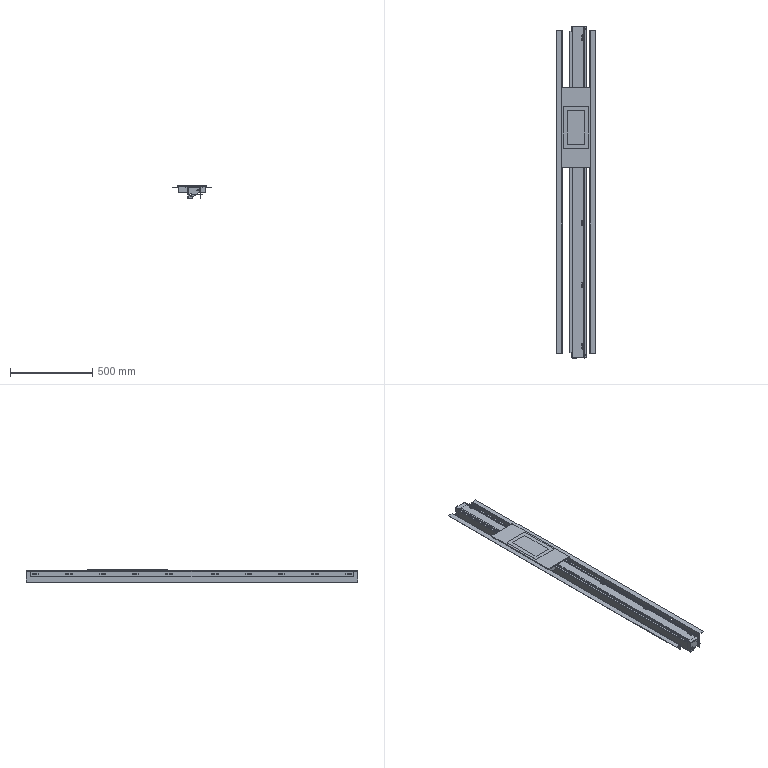Part | 14 solids | 717 faces | box 236 x 2016 x 79 mm | volume 5800115 mm3 | plane 464 | cylinder 253 | commonest cylinder face diameters 8 x60 6 x56 2 x20 9 x18 3.6 x12 10 x12